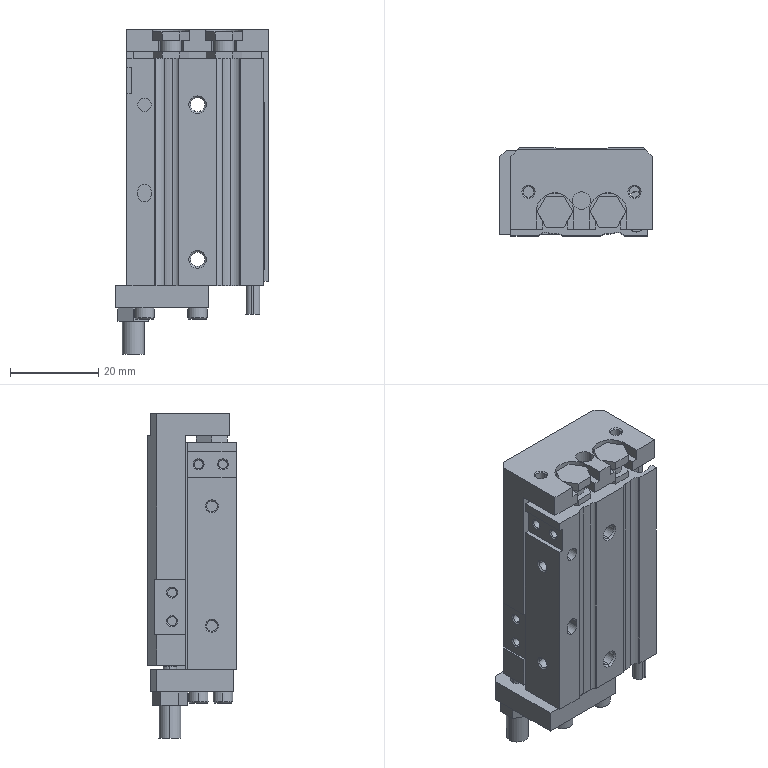Part | SolidWorks | features AEMSimFeature 1 | 5 solids | 405 faces | box 34.5 x 20 x 73.5 mm | volume 32210 mm3 | plane 228 | cylinder 131 | cone 44 | spline 2 | commonest cylinder face diameters 3 x22 2.013 x16 2.459 x16 6 x9 4.5 x8 2.1 x6